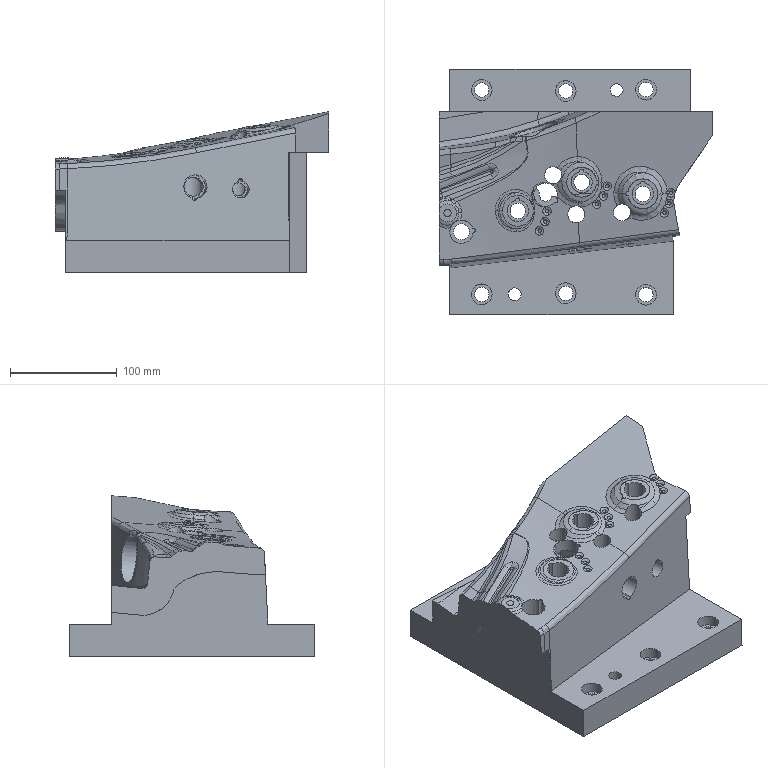Part | NX | features solid 2 | 1 solid | 225 faces | volume 3527498 mm3 | spline 99 | cylinder 69 | plane 42 | sphere 9 | torus 6 | commonest cylinder face diameters 4 x14 13.5 x6 16 x6 19.5 x6 12 x4 20 x4